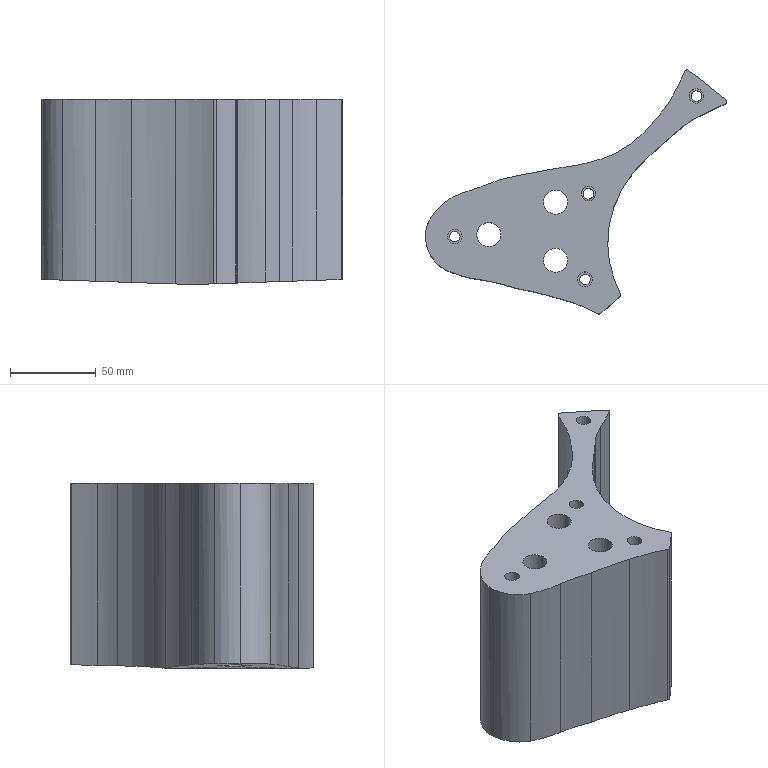Part | NX | features 8 2 | 1 solid | 51 faces | box 175.754 x 142.388 x 108 mm | volume 771641 mm3 | cylinder 37 | plane 14 | commonest cylinder face diameters 3 x4 6.2 x4 8.5 x4 14.1 x3 20 x3 40.451 x1
STEP:
#1=CARTESIAN_POINT('',(739.823,139.747,91.));
#2=VERTEX_POINT('',#1);
#3=CARTESIAN_POINT('',(732.773,139.747,91.));
#4=DIRECTION('',(0.,0.,1.));
#5=DIRECTION('',(1.,0.,0.));
#6=AXIS2_PLACEMENT_3D('',#3,#4,#5);
#7=CIRCLE('',#6,7.05);
#8=EDGE_CURVE('',#2,#2,#7,.T.);
#9=ORIENTED_EDGE('',*,*,#8,.F.);
#10=EDGE_LOOP('',(#9));
#11=FACE_BOUND('',#10,.T.);
#12=CARTESIAN_POINT('',(661.244,132.571,91.));
#13=VERTEX_POINT('',#12);
#14=CARTESIAN_POINT('',(656.895,117.671,91.));
#15=VERTEX_POINT('',#14);
#16=CARTESIAN_POINT('',(676.999,119.888,91.));
#17=DIRECTION('',(0.,0.,1.));
#18=DIRECTION('',(1.,0.,0.));
#19=AXIS2_PLACEMENT_3D('',#16,#17,#18);
#20=CIRCLE('',#19,20.225);
#21=EDGE_CURVE('',#13,#15,#20,.T.);
#22=ORIENTED_EDGE('',*,*,#21,.T.);
#23=CARTESIAN_POINT('',(669.269,99.827,91.));
#24=VERTEX_POINT('',#23);
#25=CARTESIAN_POINT('',(678.925,119.735,91.));
#26=DIRECTION('',(0.,0.,1.));
#27=DIRECTION('',(1.,0.,0.));
#28=AXIS2_PLACEMENT_3D('',#25,#26,#27);
#29=CIRCLE('',#28,22.127);
#30=EDGE_CURVE('',#15,#24,#29,.T.);
#31=ORIENTED_EDGE('',*,*,#30,.T.);
#32=CARTESIAN_POINT('',(688.554,94.53,91.));
#33=VERTEX_POINT('',#32);
#34=CARTESIAN_POINT('',(695.454,157.414,91.));
#35=DIRECTION('',(0.,0.,1.));
#36=DIRECTION('',(1.,0.,0.));
#37=AXIS2_PLACEMENT_3D('',#34,#35,#36);
#38=CIRCLE('',#37,63.261);
#39=EDGE_CURVE('',#24,#33,#38,.T.);
#40=ORIENTED_EDGE('',*,*,#39,.T.);
#41=CARTESIAN_POINT('',(709.333,89.489,91.));
#42=VERTEX_POINT('',#41);
#43=CARTESIAN_POINT('',(668.152,-34.909,91.));
#44=DIRECTION('',(0.,0.,-1.));
#45=DIRECTION('',(1.,0.,0.));
#46=AXIS2_PLACEMENT_3D('',#43,#44,#45);
#47=CIRCLE('',#46,131.038);
#48=EDGE_CURVE('',#33,#42,#47,.T.);
#49=ORIENTED_EDGE('',*,*,#48,.T.);
#50=CARTESIAN_POINT('',(734.802,83.424,91.));
#51=VERTEX_POINT('',#50);
#52=CARTESIAN_POINT('',(672.24,-122.755,91.));
#53=DIRECTION('',(0.,0.,-1.));
#54=DIRECTION('',(1.,0.,0.));
#55=AXIS2_PLACEMENT_3D('',#52,#53,#54);
#56=CIRCLE('',#55,215.461);
#57=EDGE_CURVE('',#42,#51,#56,.T.);
#58=ORIENTED_EDGE('',*,*,#57,.T.);
#59=CARTESIAN_POINT('',(757.492,74.697,91.));
#60=VERTEX_POINT('',#59);
#61=CARTESIAN_POINT('',(709.102,-17.264,91.));
#62=DIRECTION('',(0.,0.,-1.));
#63=DIRECTION('',(1.,0.,0.));
#64=AXIS2_PLACEMENT_3D('',#61,#62,#63);
#65=CIRCLE('',#64,103.916);
#66=EDGE_CURVE('',#51,#60,#65,.T.);
#67=ORIENTED_EDGE('',*,*,#66,.T.);
#68=CARTESIAN_POINT('',(759.172,74.89,91.));
#69=VERTEX_POINT('',#68);
#70=CARTESIAN_POINT('',(758.191,76.024,91.));
#71=DIRECTION('',(0.,0.,1.));
#72=DIRECTION('',(1.,0.,0.));
#73=AXIS2_PLACEMENT_3D('',#70,#71,#72);
#74=CIRCLE('',#73,1.5);
#75=EDGE_CURVE('',#60,#69,#74,.T.);
#76=ORIENTED_EDGE('',*,*,#75,.T.);
#77=CARTESIAN_POINT('',(770.213,84.446,91.));
#78=VERTEX_POINT('',#77);
#79=CARTESIAN_POINT('',(406.095,-230.692,91.));
#80=DIRECTION('',(0.7561,0.6544,0.));
#81=VECTOR('',#80,1000.);
#82=LINE('',#79,#81);
#83=EDGE_CURVE('',#69,#78,#82,.T.);
#84=ORIENTED_EDGE('',*,*,#83,.T.);
#85=CARTESIAN_POINT('',(770.56,86.277,91.));
#86=VERTEX_POINT('',#85);
#87=CARTESIAN_POINT('',(769.232,85.58,91.));
#88=DIRECTION('',(0.,0.,1.));
#89=DIRECTION('',(1.,0.,0.));
#90=AXIS2_PLACEMENT_3D('',#87,#88,#89);
#91=CIRCLE('',#90,1.5);
#92=EDGE_CURVE('',#78,#86,#91,.T.);
#93=ORIENTED_EDGE('',*,*,#92,.T.);
#94=CARTESIAN_POINT('',(763.173,114.849,91.));
#95=VERTEX_POINT('',#94);
#96=CARTESIAN_POINT('',(827.93,116.35,91.));
#97=DIRECTION('',(0.,0.,-1.));
#98=DIRECTION('',(1.,0.,0.));
#99=AXIS2_PLACEMENT_3D('',#96,#97,#98);
#100=CIRCLE('',#99,64.774);
#101=EDGE_CURVE('',#86,#95,#100,.T.);
#102=ORIENTED_EDGE('',*,*,#101,.T.);
#103=CARTESIAN_POINT('',(771.435,147.148,91.));
#104=VERTEX_POINT('',#103);
#105=CARTESIAN_POINT('',(826.446,115.87,91.));
#106=DIRECTION('',(0.,0.,-1.));
#107=DIRECTION('',(1.,0.,0.));
#108=AXIS2_PLACEMENT_3D('',#105,#106,#107);
#109=CIRCLE('',#108,63.281);
#110=EDGE_CURVE('',#95,#104,#109,.T.);
#111=ORIENTED_EDGE('',*,*,#110,.T.);
#112=CARTESIAN_POINT('',(787.822,167.002,91.));
#113=VERTEX_POINT('',#112);
#114=CARTESIAN_POINT('',(839.48,107.677,91.));
#115=DIRECTION('',(0.,0.,-1.));
#116=DIRECTION('',(1.,0.,0.));
#117=AXIS2_PLACEMENT_3D('',#114,#115,#116);
#118=CIRCLE('',#117,78.664);
#119=EDGE_CURVE('',#104,#113,#118,.T.);
#120=ORIENTED_EDGE('',*,*,#119,.T.);
#121=CARTESIAN_POINT('',(795.884,174.026,91.));
#122=VERTEX_POINT('',#121);
#123=CARTESIAN_POINT('',(374.973,-192.67,91.));
#124=DIRECTION('',(0.754,0.6569,0.));
#125=VECTOR('',#124,1000.);
#126=LINE('',#123,#125);
#127=EDGE_CURVE('',#113,#122,#126,.T.);
#128=ORIENTED_EDGE('',*,*,#127,.T.);
#129=CARTESIAN_POINT('',(803.49,180.68,91.));
#130=VERTEX_POINT('',#129);
#131=CARTESIAN_POINT('',(376.367,-192.972,91.));
#132=DIRECTION('',(0.7526,0.6584,0.));
#133=VECTOR('',#132,1000.);
#134=LINE('',#131,#133);
#135=EDGE_CURVE('',#122,#130,#134,.T.);
#136=ORIENTED_EDGE('',*,*,#135,.T.);
#137=CARTESIAN_POINT('',(817.08,190.116,91.));
#138=VERTEX_POINT('',#137);
#139=CARTESIAN_POINT('',(840.917,141.281,91.));
#140=DIRECTION('',(0.,0.,-1.));
#141=DIRECTION('',(1.,0.,0.));
#142=AXIS2_PLACEMENT_3D('',#139,#140,#141);
#143=CIRCLE('',#142,54.342);
#144=EDGE_CURVE('',#130,#138,#143,.T.);
#145=ORIENTED_EDGE('',*,*,#144,.T.);
#146=CARTESIAN_POINT('',(831.695,197.052,91.));
#147=VERTEX_POINT('',#146);
#148=CARTESIAN_POINT('',(632.757,597.362,91.));
#149=DIRECTION('',(0.,0.,1.));
#150=DIRECTION('',(1.,0.,0.));
#151=AXIS2_PLACEMENT_3D('',#148,#149,#150);
#152=CIRCLE('',#151,447.018);
#153=EDGE_CURVE('',#138,#147,#152,.T.);
#154=ORIENTED_EDGE('',*,*,#153,.T.);
#155=CARTESIAN_POINT('',(831.961,199.569,91.));
#156=VERTEX_POINT('',#155);
#157=CARTESIAN_POINT('',(831.027,198.395,91.));
#158=DIRECTION('',(0.,0.,1.));
#159=DIRECTION('',(1.,0.,0.));
#160=AXIS2_PLACEMENT_3D('',#157,#158,#159);
#161=CIRCLE('',#160,1.5);
#162=EDGE_CURVE('',#147,#156,#161,.T.);
#163=ORIENTED_EDGE('',*,*,#162,.T.);
#164=CARTESIAN_POINT('',(810.569,216.587,91.));
#165=VERTEX_POINT('',#164);
#166=CARTESIAN_POINT('',(424.096,524.034,91.));
#167=DIRECTION('',(-0.7826,0.6226,0.));
#168=VECTOR('',#167,1000.);
#169=LINE('',#166,#168);
#170=EDGE_CURVE('',#156,#165,#169,.T.);
#171=ORIENTED_EDGE('',*,*,#170,.T.);
#172=CARTESIAN_POINT('',(808.272,216.04,91.));
#173=VERTEX_POINT('',#172);
#174=CARTESIAN_POINT('',(809.635,215.413,91.));
#175=DIRECTION('',(0.,0.,1.));
#176=DIRECTION('',(1.,0.,0.));
#177=AXIS2_PLACEMENT_3D('',#174,#175,#176);
#178=CIRCLE('',#177,1.5);
#179=EDGE_CURVE('',#165,#173,#178,.T.);
#180=ORIENTED_EDGE('',*,*,#179,.T.);
#181=CARTESIAN_POINT('',(800.673,201.002,91.));
#182=VERTEX_POINT('',#181);
#183=CARTESIAN_POINT('',(597.133,313.29,91.));
#184=DIRECTION('',(0.,0.,-1.));
#185=DIRECTION('',(1.,0.,0.));
#186=AXIS2_PLACEMENT_3D('',#183,#184,#185);
#187=CIRCLE('',#186,232.459);
#188=EDGE_CURVE('',#173,#182,#187,.T.);
#189=ORIENTED_EDGE('',*,*,#188,.T.);
#190=CARTESIAN_POINT('',(792.153,189.249,91.));
#191=VERTEX_POINT('',#190);
#192=CARTESIAN_POINT('',(742.965,233.873,91.));
#193=DIRECTION('',(0.,0.,-1.));
#194=DIRECTION('',(1.,0.,0.));
#195=AXIS2_PLACEMENT_3D('',#192,#193,#194);
#196=CIRCLE('',#195,66.413);
#197=EDGE_CURVE('',#182,#191,#196,.T.);
#198=ORIENTED_EDGE('',*,*,#197,.T.);
#199=CARTESIAN_POINT('',(767.073,167.853,91.));
#200=VERTEX_POINT('',#199);
#201=CARTESIAN_POINT('',(735.807,229.9,91.));
#202=DIRECTION('',(0.,0.,-1.));
#203=DIRECTION('',(1.,0.,0.));
#204=AXIS2_PLACEMENT_3D('',#201,#202,#203);
#205=CIRCLE('',#204,69.48);
#206=EDGE_CURVE('',#191,#200,#205,.T.);
#207=ORIENTED_EDGE('',*,*,#206,.T.);
#208=CARTESIAN_POINT('',(744.942,161.237,91.));
#209=VERTEX_POINT('',#208);
#210=CARTESIAN_POINT('',(729.089,254.594,91.));
#211=DIRECTION('',(0.,0.,-1.));
#212=DIRECTION('',(1.,0.,0.));
#213=AXIS2_PLACEMENT_3D('',#210,#211,#212);
#214=CIRCLE('',#213,94.693);
#215=EDGE_CURVE('',#200,#209,#214,.T.);
#216=ORIENTED_EDGE('',*,*,#215,.T.);
#217=CARTESIAN_POINT('',(699.905,152.757,91.));
#218=VERTEX_POINT('',#217);
#219=CARTESIAN_POINT('',(820.799,-365.438,91.));
#220=DIRECTION('',(0.,0.,1.));
#221=DIRECTION('',(1.,0.,0.));
#222=AXIS2_PLACEMENT_3D('',#219,#220,#221);
#223=CIRCLE('',#222,532.11);
#224=EDGE_CURVE('',#209,#218,#223,.T.);
#225=ORIENTED_EDGE('',*,*,#224,.T.);
#226=CARTESIAN_POINT('',(680.986,145.908,91.));
#227=VERTEX_POINT('',#226);
#228=CARTESIAN_POINT('',(585.955,437.965,91.));
#229=DIRECTION('',(0.,0.,-1.));
#230=DIRECTION('',(1.,0.,0.));
#231=AXIS2_PLACEMENT_3D('',#228,#229,#230);
#232=CIRCLE('',#231,307.129);
#233=EDGE_CURVE('',#218,#227,#232,.T.);
#234=ORIENTED_EDGE('',*,*,#233,.T.);
#235=CARTESIAN_POINT('',(671.706,142.125,91.));
#236=VERTEX_POINT('',#235);
#237=CARTESIAN_POINT('',(693.196,102.677,91.));
#238=DIRECTION('',(0.,0.,1.));
#239=DIRECTION('',(1.,0.,0.));
#240=AXIS2_PLACEMENT_3D('',#237,#238,#239);
#241=CIRCLE('',#240,44.922);
#242=EDGE_CURVE('',#227,#236,#241,.T.);
#243=ORIENTED_EDGE('',*,*,#242,.T.);
#244=CARTESIAN_POINT('',(691.977,109.423,91.));
#245=DIRECTION('',(0.,0.,1.));
#246=DIRECTION('',(1.,0.,0.));
#247=AXIS2_PLACEMENT_3D('',#244,#245,#246);
#248=CIRCLE('',#247,38.475);
#249=EDGE_CURVE('',#236,#13,#248,.T.);
#250=ORIENTED_EDGE('',*,*,#249,.T.);
#251=EDGE_LOOP('',(#22,#31,#40,#49,#58,#67,#76,#84,#93,#102,#111,#120,#128,#136,#145,#154,#163,#171,#180,#189,#198,#207,#216,#225,#234,#243,#250));
#252=FACE_BOUND('',#251,.T.);
#253=CARTESIAN_POINT('',(678.189,119.723,91.));
#254=VERTEX_POINT('',#253);
#255=CARTESIAN_POINT('',(673.939,119.723,91.));
#256=DIRECTION('',(0.,0.,-1.));
#257=DIRECTION('',(1.,0.,0.));
#258=AXIS2_PLACEMENT_3D('',#255,#256,#257);
#259=CIRCLE('',#258,4.25);
#260=EDGE_CURVE('',#254,#254,#259,.T.);
#261=ORIENTED_EDGE('',*,*,#260,.T.);
#262=EDGE_LOOP('',(#261));
#263=FACE_BOUND('',#262,.T.);
#264=CARTESIAN_POINT('',(754.189,94.723,91.));
#265=VERTEX_POINT('',#264);
#266=CARTESIAN_POINT('',(749.939,94.723,91.));
#267=DIRECTION('',(0.,0.,-1.));
#268=DIRECTION('',(1.,0.,0.));
#269=AXIS2_PLACEMENT_3D('',#266,#267,#268);
#270=CIRCLE('',#269,4.25);
#271=EDGE_CURVE('',#265,#265,#270,.T.);
#272=ORIENTED_EDGE('',*,*,#271,.T.);
#273=EDGE_LOOP('',(#272));
#274=FACE_BOUND('',#273,.T.);
#275=CARTESIAN_POINT('',(756.189,144.723,91.));
#276=VERTEX_POINT('',#275);
#277=CARTESIAN_POINT('',(751.939,144.723,91.));
#278=DIRECTION('',(0.,0.,-1.));
#279=DIRECTION('',(1.,0.,0.));
#280=AXIS2_PLACEMENT_3D('',#277,#278,#279);
#281=CIRCLE('',#280,4.25);
#282=EDGE_CURVE('',#276,#276,#281,.T.);
#283=ORIENTED_EDGE('',*,*,#282,.T.);
#284=EDGE_LOOP('',(#283));
#285=FACE_BOUND('',#284,.T.);
#286=CARTESIAN_POINT('',(819.189,201.723,91.));
#287=VERTEX_POINT('',#286);
#288=CARTESIAN_POINT('',(814.939,201.723,91.));
#289=DIRECTION('',(0.,0.,-1.));
#290=DIRECTION('',(1.,0.,0.));
#291=AXIS2_PLACEMENT_3D('',#288,#289,#290);
#292=CIRCLE('',#291,4.25);
#293=EDGE_CURVE('',#287,#287,#292,.T.);
#294=ORIENTED_EDGE('',*,*,#293,.T.);
#295=EDGE_LOOP('',(#294));
#296=FACE_BOUND('',#295,.T.);
#297=CARTESIAN_POINT('',(739.823,105.747,91.));
#298=VERTEX_POINT('',#297);
#299=CARTESIAN_POINT('',(732.773,105.747,91.));
#300=DIRECTION('',(0.,0.,1.));
#301=DIRECTION('',(1.,0.,0.));
#302=AXIS2_PLACEMENT_3D('',#299,#300,#301);
#303=CIRCLE('',#302,7.05);
#304=EDGE_CURVE('',#298,#298,#303,.T.);
#305=ORIENTED_EDGE('',*,*,#304,.F.);
#306=EDGE_LOOP('',(#305));
#307=FACE_BOUND('',#306,.T.);
#308=CARTESIAN_POINT('',(700.823,120.747,91.));
#309=VERTEX_POINT('',#308);
#310=CARTESIAN_POINT('',(693.773,120.747,91.));
#311=DIRECTION('',(0.,0.,1.));
#312=DIRECTION('',(1.,0.,0.));
#313=AXIS2_PLACEMENT_3D('',#310,#311,#312);
#314=CIRCLE('',#313,7.05);
#315=EDGE_CURVE('',#309,#309,#314,.T.);
#316=ORIENTED_EDGE('',*,*,#315,.F.);
#317=EDGE_LOOP('',(#316));
#318=FACE_BOUND('',#317,.T.);
#319=CARTESIAN_POINT('',(102.63,119.939,91.));
#320=DIRECTION('',(0.,0.,1.));
#321=DIRECTION('',(-1.,0.,0.));
#322=AXIS2_PLACEMENT_3D('',#319,#320,#321);
#323=PLANE('',#322);
#324=ADVANCED_FACE('',(#11,#252,#263,#274,#285,#296,#307,#318),#323,.T.);
#325=CARTESIAN_POINT('',(683.773,120.747,-14.918));
#326=VERTEX_POINT('',#325);
#327=CARTESIAN_POINT('',(693.773,120.747,-15.258));
#328=DIRECTION('',(-0.03397,0.,-0.9994));
#329=DIRECTION('',(-0.9994,0.,0.03397));
#330=AXIS2_PLACEMENT_3D('',#327,#328,#329);
#331=ELLIPSE('',#330,10.006,10.);
#332=EDGE_CURVE('',#326,#326,#331,.T.);
#333=ORIENTED_EDGE('',*,*,#332,.F.);
#334=EDGE_LOOP('',(#333));
#335=FACE_BOUND('',#334,.T.);
#336=CARTESIAN_POINT('',(722.773,139.747,-16.243));
#337=VERTEX_POINT('',#336);
#338=CARTESIAN_POINT('',(732.773,139.747,-16.583));
#339=DIRECTION('',(-0.03397,0.,-0.9994));
#340=DIRECTION('',(-0.9994,0.,0.03397));
#341=AXIS2_PLACEMENT_3D('',#338,#339,#340);
#342=ELLIPSE('',#341,10.006,10.);
#343=EDGE_CURVE('',#337,#337,#342,.T.);
#344=ORIENTED_EDGE('',*,*,#343,.F.);
#345=EDGE_LOOP('',(#344));
#346=FACE_BOUND('',#345,.T.);
#347=CARTESIAN_POINT('',(722.773,105.747,-16.243));
#348=VERTEX_POINT('',#347);
#349=CARTESIAN_POINT('',(732.773,105.747,-16.583));
#350=DIRECTION('',(-0.03397,0.,-0.9994));
#351=DIRECTION('',(-0.9994,0.,0.03397));
#352=AXIS2_PLACEMENT_3D('',#349,#350,#351);
#353=ELLIPSE('',#352,10.006,10.);
#354=EDGE_CURVE('',#348,#348,#353,.T.);
#355=ORIENTED_EDGE('',*,*,#354,.F.);
#356=EDGE_LOOP('',(#355));
#357=FACE_BOUND('',#356,.T.);
#358=CARTESIAN_POINT('',(677.039,119.723,-14.689));
#359=VERTEX_POINT('',#358);
#360=CARTESIAN_POINT('',(673.939,119.723,-14.583));
#361=DIRECTION('',(-0.03397,0.,-0.9994));
#362=DIRECTION('',(0.9994,0.,-0.03397));
#363=AXIS2_PLACEMENT_3D('',#360,#361,#362);
#364=ELLIPSE('',#363,3.102,3.1);
#365=EDGE_CURVE('',#359,#359,#364,.T.);
#366=ORIENTED_EDGE('',*,*,#365,.F.);
#367=EDGE_LOOP('',(#366));
#368=FACE_BOUND('',#367,.T.);
#369=CARTESIAN_POINT('',(744.942,161.237,-16.997));
#370=VERTEX_POINT('',#369);
#371=CARTESIAN_POINT('',(745.033,161.253,-17.));
#372=VERTEX_POINT('',#371);
#373=CARTESIAN_POINT('',(729.089,254.594,-16.458));
#374=DIRECTION('',(0.03397,0.,0.9994));
#375=DIRECTION('',(0.9994,0.,-0.03397));
#376=AXIS2_PLACEMENT_3D('',#373,#374,#375);
#377=ELLIPSE('',#376,94.747,94.693);
#378=EDGE_CURVE('',#370,#372,#377,.T.);
#379=ORIENTED_EDGE('',*,*,#378,.T.);
#380=CARTESIAN_POINT('',(745.033,80.242,-17.));
#381=VERTEX_POINT('',#380);
#382=CARTESIAN_POINT('',(745.033,120.747,-17.));
#383=DIRECTION('',(0.,-1.,0.));
#384=VECTOR('',#383,1000.);
#385=LINE('',#382,#384);
#386=EDGE_CURVE('',#372,#381,#385,.T.);
#387=ORIENTED_EDGE('',*,*,#386,.T.);
#388=CARTESIAN_POINT('',(734.802,83.424,-16.652));
#389=VERTEX_POINT('',#388);
#390=CARTESIAN_POINT('',(709.102,-17.264,-15.779));
#391=DIRECTION('',(0.03397,0.,0.9994));
#392=DIRECTION('',(0.9994,0.,-0.03397));
#393=AXIS2_PLACEMENT_3D('',#390,#391,#392);
#394=ELLIPSE('',#393,103.976,103.916);
#395=EDGE_CURVE('',#381,#389,#394,.T.);
#396=ORIENTED_EDGE('',*,*,#395,.T.);
#397=CARTESIAN_POINT('',(709.333,89.489,-15.787));
#398=VERTEX_POINT('',#397);
#399=CARTESIAN_POINT('',(672.24,-122.755,-14.526));
#400=DIRECTION('',(0.03397,0.,0.9994));
#401=DIRECTION('',(0.9994,0.,-0.03397));
#402=AXIS2_PLACEMENT_3D('',#399,#400,#401);
#403=ELLIPSE('',#402,215.585,215.461);
#404=EDGE_CURVE('',#389,#398,#403,.T.);
#405=ORIENTED_EDGE('',*,*,#404,.T.);
#406=CARTESIAN_POINT('',(688.554,94.53,-15.08));
#407=VERTEX_POINT('',#406);
#408=CARTESIAN_POINT('',(668.152,-34.909,-14.387));
#409=DIRECTION('',(0.03397,0.,0.9994));
#410=DIRECTION('',(0.9994,0.,-0.03397));
#411=AXIS2_PLACEMENT_3D('',#408,#409,#410);
#412=ELLIPSE('',#411,131.114,131.038);
#413=EDGE_CURVE('',#398,#407,#412,.T.);
#414=ORIENTED_EDGE('',*,*,#413,.T.);
#415=CARTESIAN_POINT('',(669.269,99.827,-14.425));
#416=VERTEX_POINT('',#415);
#417=CARTESIAN_POINT('',(695.454,157.414,-15.315));
#418=DIRECTION('',(0.03397,0.,0.9994));
#419=DIRECTION('',(0.9994,0.,-0.03397));
#420=AXIS2_PLACEMENT_3D('',#417,#418,#419);
#421=ELLIPSE('',#420,63.297,63.261);
#422=EDGE_CURVE('',#416,#407,#421,.T.);
#423=ORIENTED_EDGE('',*,*,#422,.F.);
#424=CARTESIAN_POINT('',(656.895,117.671,-14.004));
#425=VERTEX_POINT('',#424);
#426=CARTESIAN_POINT('',(678.925,119.735,-14.753));
#427=DIRECTION('',(0.03397,0.,0.9994));
#428=DIRECTION('',(0.9994,0.,-0.03397));
#429=AXIS2_PLACEMENT_3D('',#426,#427,#428);
#430=ELLIPSE('',#429,22.139,22.127);
#431=EDGE_CURVE('',#425,#416,#430,.T.);
#432=ORIENTED_EDGE('',*,*,#431,.F.);
#433=CARTESIAN_POINT('',(661.244,132.571,-14.152));
#434=VERTEX_POINT('',#433);
#435=CARTESIAN_POINT('',(676.999,119.888,-14.687));
#436=DIRECTION('',(0.03397,0.,0.9994));
#437=DIRECTION('',(0.9994,0.,-0.03397));
#438=AXIS2_PLACEMENT_3D('',#435,#436,#437);
#439=ELLIPSE('',#438,20.237,20.225);
#440=EDGE_CURVE('',#434,#425,#439,.T.);
#441=ORIENTED_EDGE('',*,*,#440,.F.);
#442=CARTESIAN_POINT('',(671.706,142.125,-14.508));
#443=VERTEX_POINT('',#442);
#444=CARTESIAN_POINT('',(691.977,109.423,-15.197));
#445=DIRECTION('',(0.03397,0.,0.9994));
#446=DIRECTION('',(0.9994,0.,-0.03397));
#447=AXIS2_PLACEMENT_3D('',#444,#445,#446);
#448=ELLIPSE('',#447,38.497,38.475);
#449=EDGE_CURVE('',#443,#434,#448,.T.);
#450=ORIENTED_EDGE('',*,*,#449,.F.);
#451=CARTESIAN_POINT('',(680.986,145.908,-14.823));
#452=VERTEX_POINT('',#451);
#453=CARTESIAN_POINT('',(693.196,102.677,-15.238));
#454=DIRECTION('',(0.03397,0.,0.9994));
#455=DIRECTION('',(0.9994,0.,-0.03397));
#456=AXIS2_PLACEMENT_3D('',#453,#454,#455);
#457=ELLIPSE('',#456,44.948,44.922);
#458=EDGE_CURVE('',#452,#443,#457,.T.);
#459=ORIENTED_EDGE('',*,*,#458,.F.);
#460=CARTESIAN_POINT('',(699.905,152.757,-15.466));
#461=VERTEX_POINT('',#460);
#462=CARTESIAN_POINT('',(585.955,437.965,-11.593));
#463=DIRECTION('',(0.03397,0.,0.9994));
#464=DIRECTION('',(0.9994,0.,-0.03397));
#465=AXIS2_PLACEMENT_3D('',#462,#463,#464);
#466=ELLIPSE('',#465,307.307,307.129);
#467=EDGE_CURVE('',#452,#461,#466,.T.);
#468=ORIENTED_EDGE('',*,*,#467,.T.);
#469=CARTESIAN_POINT('',(820.799,-365.438,-19.575));
#470=DIRECTION('',(0.03397,0.,0.9994));
#471=DIRECTION('',(0.9994,0.,-0.03397));
#472=AXIS2_PLACEMENT_3D('',#469,#470,#471);
#473=ELLIPSE('',#472,532.417,532.11);
#474=EDGE_CURVE('',#370,#461,#473,.T.);
#475=ORIENTED_EDGE('',*,*,#474,.F.);
#476=EDGE_LOOP('',(#379,#387,#396,#405,#414,#423,#432,#441,#450,#459,#468,#475));
#477=FACE_BOUND('',#476,.T.);
#478=CARTESIAN_POINT('',(700.903,120.747,-15.5));
#479=DIRECTION('',(-0.03397,0.,-0.9994));
#480=DIRECTION('',(0.9994,0.,-0.03397));
#481=AXIS2_PLACEMENT_3D('',#478,#479,#480);
#482=PLANE('',#481);
#483=ADVANCED_FACE('',(#335,#346,#357,#368,#477),#482,.T.);
#484=CARTESIAN_POINT('',(757.492,74.697,-16.576));
#485=VERTEX_POINT('',#484);
#486=CARTESIAN_POINT('',(709.102,-17.264,-18.221));
#487=DIRECTION('',(-0.03397,0.,0.9994));
#488=DIRECTION('',(-0.9994,0.,-0.03397));
#489=AXIS2_PLACEMENT_3D('',#486,#487,#488);
#490=ELLIPSE('',#489,103.976,103.916);
#491=EDGE_CURVE('',#485,#381,#490,.T.);
#492=ORIENTED_EDGE('',*,*,#491,.F.);
#493=CARTESIAN_POINT('',(757.492,74.697,16.));
#494=DIRECTION('',(0.,0.,-1.));
#495=VECTOR('',#494,1000.);
#496=LINE('',#493,#495);
#497=EDGE_CURVE('',#60,#485,#496,.T.);
#498=ORIENTED_EDGE('',*,*,#497,.F.);
#499=ORIENTED_EDGE('',*,*,#66,.F.);
#500=CARTESIAN_POINT('',(734.802,83.424,16.));
#501=DIRECTION('',(0.,0.,-1.));
#502=VECTOR('',#501,1000.);
#503=LINE('',#500,#502);
#504=EDGE_CURVE('',#51,#389,#503,.T.);
#505=ORIENTED_EDGE('',*,*,#504,.T.);
#506=ORIENTED_EDGE('',*,*,#395,.F.);
#507=EDGE_LOOP('',(#492,#498,#499,#505,#506));
#508=FACE_BOUND('',#507,.T.);
#509=CARTESIAN_POINT('',(709.102,-17.264,16.));
#510=DIRECTION('',(0.,0.,-1.));
#511=DIRECTION('',(-1.,0.,0.));
#512=AXIS2_PLACEMENT_3D('',#509,#510,#511);
#513=CYLINDRICAL_SURFACE('',#512,103.916);
#514=ADVANCED_FACE('',(#508),#513,.F.);
#515=ORIENTED_EDGE('',*,*,#497,.T.);
#516=CARTESIAN_POINT('',(759.172,74.89,-16.519));
#517=VERTEX_POINT('',#516);
#518=CARTESIAN_POINT('',(758.191,76.024,-16.553));
#519=DIRECTION('',(-0.03397,0.,0.9994));
#520=DIRECTION('',(-0.9994,0.,-0.03397));
#521=AXIS2_PLACEMENT_3D('',#518,#519,#520);
#522=ELLIPSE('',#521,1.501,1.5);
#523=EDGE_CURVE('',#485,#517,#522,.T.);
#524=ORIENTED_EDGE('',*,*,#523,.T.);
#525=CARTESIAN_POINT('',(759.172,74.89,16.));
#526=DIRECTION('',(0.,0.,-1.));
#527=VECTOR('',#526,1000.);
#528=LINE('',#525,#527);
#529=EDGE_CURVE('',#69,#517,#528,.T.);
#530=ORIENTED_EDGE('',*,*,#529,.F.);
#531=ORIENTED_EDGE('',*,*,#75,.F.);
#532=EDGE_LOOP('',(#515,#524,#530,#531));
#533=FACE_BOUND('',#532,.T.);
#534=CARTESIAN_POINT('',(758.191,76.024,16.));
#535=DIRECTION('',(0.,0.,-1.));
#536=DIRECTION('',(-1.,0.,0.));
#537=AXIS2_PLACEMENT_3D('',#534,#535,#536);
#538=CYLINDRICAL_SURFACE('',#537,1.5);
#539=ADVANCED_FACE('',(#533),#538,.T.);
#540=CARTESIAN_POINT('',(770.213,84.446,-16.144));
#541=VERTEX_POINT('',#540);
#542=CARTESIAN_POINT('',(759.707,75.353,-16.501));
#543=DIRECTION('',(-0.7559,-0.6542,-0.02569));
#544=VECTOR('',#543,1000.);
#545=LINE('',#542,#544);
#546=EDGE_CURVE('',#541,#517,#545,.T.);
#547=ORIENTED_EDGE('',*,*,#546,.F.);
#548=CARTESIAN_POINT('',(770.213,84.446,16.));
#549=DIRECTION('',(0.,0.,-1.));
#550=VECTOR('',#549,1000.);
#551=LINE('',#548,#550);
#552=EDGE_CURVE('',#78,#541,#551,.T.);
#553=ORIENTED_EDGE('',*,*,#552,.F.);
#554=ORIENTED_EDGE('',*,*,#83,.F.);
#555=ORIENTED_EDGE('',*,*,#529,.T.);
#556=EDGE_LOOP('',(#547,#553,#554,#555));
#557=FACE_BOUND('',#556,.T.);
#558=CARTESIAN_POINT('',(759.172,74.89,16.));
#559=DIRECTION('',(-0.6544,0.7561,0.));
#560=DIRECTION('',(-0.7561,-0.6544,0.));
#561=AXIS2_PLACEMENT_3D('',#558,#559,#560);
#562=PLANE('',#561);
#563=ADVANCED_FACE('',(#557),#562,.F.);
#564=ORIENTED_EDGE('',*,*,#552,.T.);
#565=CARTESIAN_POINT('',(770.56,86.277,-16.132));
#566=VERTEX_POINT('',#565);
#567=CARTESIAN_POINT('',(769.232,85.58,-16.177));
#568=DIRECTION('',(-0.03397,0.,0.9994));
#569=DIRECTION('',(-0.9994,0.,-0.03397));
#570=AXIS2_PLACEMENT_3D('',#567,#568,#569);
#571=ELLIPSE('',#570,1.501,1.5);
#572=EDGE_CURVE('',#541,#566,#571,.T.);
#573=ORIENTED_EDGE('',*,*,#572,.T.);
#574=CARTESIAN_POINT('',(770.56,86.277,16.));
#575=DIRECTION('',(0.,0.,-1.));
#576=VECTOR('',#575,1000.);
#577=LINE('',#574,#576);
#578=EDGE_CURVE('',#86,#566,#577,.T.);
#579=ORIENTED_EDGE('',*,*,#578,.F.);
#580=ORIENTED_EDGE('',*,*,#92,.F.);
#581=EDGE_LOOP('',(#564,#573,#579,#580));
#582=FACE_BOUND('',#581,.T.);
#583=CARTESIAN_POINT('',(769.232,85.58,16.));
#584=DIRECTION('',(0.,0.,-1.));
#585=DIRECTION('',(-1.,0.,0.));
#586=AXIS2_PLACEMENT_3D('',#583,#584,#585);
#587=CYLINDRICAL_SURFACE('',#586,1.5);
#588=ADVANCED_FACE('',(#582),#587,.T.);
#589=CARTESIAN_POINT('',(763.173,114.849,-16.383));
#590=VERTEX_POINT('',#589);
#591=CARTESIAN_POINT('',(827.93,116.35,-14.182));
#592=DIRECTION('',(-0.03397,0.,0.9994));
#593=DIRECTION('',(-0.9994,0.,-0.03397));
#594=AXIS2_PLACEMENT_3D('',#591,#592,#593);
#595=ELLIPSE('',#594,64.811,64.774);
#596=EDGE_CURVE('',#590,#566,#595,.T.);
#597=ORIENTED_EDGE('',*,*,#596,.F.);
#598=CARTESIAN_POINT('',(763.173,114.849,16.));
#599=DIRECTION('',(0.,0.,-1.));
#600=VECTOR('',#599,1000.);
#601=LINE('',#598,#600);
#602=EDGE_CURVE('',#95,#590,#601,.T.);
#603=ORIENTED_EDGE('',*,*,#602,.F.);
#604=ORIENTED_EDGE('',*,*,#101,.F.);
#605=ORIENTED_EDGE('',*,*,#578,.T.);
#606=EDGE_LOOP('',(#597,#603,#604,#605));
#607=FACE_BOUND('',#606,.T.);
#608=CARTESIAN_POINT('',(827.93,116.35,16.));
#609=DIRECTION('',(0.,0.,-1.));
#610=DIRECTION('',(-1.,0.,0.));
#611=AXIS2_PLACEMENT_3D('',#608,#609,#610);
#612=CYLINDRICAL_SURFACE('',#611,64.774);
#613=ADVANCED_FACE('',(#607),#612,.F.);
#614=CARTESIAN_POINT('',(771.435,147.148,-16.103));
#615=VERTEX_POINT('',#614);
#616=CARTESIAN_POINT('',(826.446,115.87,-14.233));
#617=DIRECTION('',(-0.03397,0.,0.9994));
#618=DIRECTION('',(-0.9994,0.,-0.03397));
#619=AXIS2_PLACEMENT_3D('',#616,#617,#618);
#620=ELLIPSE('',#619,63.318,63.281);
#621=EDGE_CURVE('',#615,#590,#620,.T.);
#622=ORIENTED_EDGE('',*,*,#621,.F.);
#623=CARTESIAN_POINT('',(771.435,147.148,16.));
#624=DIRECTION('',(0.,0.,-1.));
#625=VECTOR('',#624,1000.);
#626=LINE('',#623,#625);
#627=EDGE_CURVE('',#104,#615,#626,.T.);
#628=ORIENTED_EDGE('',*,*,#627,.F.);
#629=ORIENTED_EDGE('',*,*,#110,.F.);
#630=ORIENTED_EDGE('',*,*,#602,.T.);
#631=EDGE_LOOP('',(#622,#628,#629,#630));
#632=FACE_BOUND('',#631,.T.);
#633=CARTESIAN_POINT('',(826.446,115.87,16.));
#634=DIRECTION('',(0.,0.,-1.));
#635=DIRECTION('',(-1.,0.,0.));
#636=AXIS2_PLACEMENT_3D('',#633,#634,#635);
#637=CYLINDRICAL_SURFACE('',#636,63.281);
#638=ADVANCED_FACE('',(#632),#637,.F.);
#639=CARTESIAN_POINT('',(787.822,167.002,-15.546));
#640=VERTEX_POINT('',#639);
#641=CARTESIAN_POINT('',(839.48,107.677,-13.79));
#642=DIRECTION('',(-0.03397,0.,0.9994));
#643=DIRECTION('',(-0.9994,0.,-0.03397));
#644=AXIS2_PLACEMENT_3D('',#641,#642,#643);
#645=ELLIPSE('',#644,78.71,78.664);
#646=EDGE_CURVE('',#640,#615,#645,.T.);
#647=ORIENTED_EDGE('',*,*,#646,.F.);
#648=CARTESIAN_POINT('',(787.822,167.002,16.));
#649=DIRECTION('',(0.,0.,-1.));
#650=VECTOR('',#649,1000.);
#651=LINE('',#648,#650);
#652=EDGE_CURVE('',#113,#640,#651,.T.);
#653=ORIENTED_EDGE('',*,*,#652,.F.);
#654=ORIENTED_EDGE('',*,*,#119,.F.);
#655=ORIENTED_EDGE('',*,*,#627,.T.);
#656=EDGE_LOOP('',(#647,#653,#654,#655));
#657=FACE_BOUND('',#656,.T.);
#658=CARTESIAN_POINT('',(839.48,107.677,16.));
#659=DIRECTION('',(0.,0.,-1.));
#660=DIRECTION('',(-1.,0.,0.));
#661=AXIS2_PLACEMENT_3D('',#658,#659,#660);
#662=CYLINDRICAL_SURFACE('',#661,78.664);
#663=ADVANCED_FACE('',(#657),#662,.F.);
#664=CARTESIAN_POINT('',(795.884,174.026,-15.272));
#665=VERTEX_POINT('',#664);
#666=CARTESIAN_POINT('',(788.335,167.449,-15.528));
#667=DIRECTION('',(-0.7537,-0.6567,-0.02562));
#668=VECTOR('',#667,1000.);
#669=LINE('',#666,#668);
#670=EDGE_CURVE('',#665,#640,#669,.T.);
#671=ORIENTED_EDGE('',*,*,#670,.F.);
#672=CARTESIAN_POINT('',(795.884,174.026,16.));
#673=DIRECTION('',(0.,0.,-1.));
#674=VECTOR('',#673,1000.);
#675=LINE('',#672,#674);
#676=EDGE_CURVE('',#122,#665,#675,.T.);
#677=ORIENTED_EDGE('',*,*,#676,.F.);
#678=ORIENTED_EDGE('',*,*,#127,.F.);
#679=ORIENTED_EDGE('',*,*,#652,.T.);
#680=EDGE_LOOP('',(#671,#677,#678,#679));
#681=FACE_BOUND('',#680,.T.);
#682=CARTESIAN_POINT('',(787.822,167.002,16.));
#683=DIRECTION('',(-0.6569,0.754,0.));
#684=DIRECTION('',(-0.754,-0.6569,0.));
#685=AXIS2_PLACEMENT_3D('',#682,#683,#684);
#686=PLANE('',#685);
#687=ADVANCED_FACE('',(#681),#686,.F.);
#688=CARTESIAN_POINT('',(803.49,180.68,-15.013));
#689=VERTEX_POINT('',#688);
#690=CARTESIAN_POINT('',(796.39,174.468,-15.254));
#691=DIRECTION('',(-0.7524,-0.6582,-0.02557));
#692=VECTOR('',#691,1000.);
#693=LINE('',#690,#692);
#694=EDGE_CURVE('',#689,#665,#693,.T.);
#695=ORIENTED_EDGE('',*,*,#694,.F.);
#696=CARTESIAN_POINT('',(803.49,180.68,16.));
#697=DIRECTION('',(0.,0.,-1.));
#698=VECTOR('',#697,1000.);
#699=LINE('',#696,#698);
#700=EDGE_CURVE('',#130,#689,#699,.T.);
#701=ORIENTED_EDGE('',*,*,#700,.F.);
#702=ORIENTED_EDGE('',*,*,#135,.F.);
#703=ORIENTED_EDGE('',*,*,#676,.T.);
#704=EDGE_LOOP('',(#695,#701,#702,#703));
#705=FACE_BOUND('',#704,.T.);
#706=CARTESIAN_POINT('',(795.884,174.026,16.));
#707=DIRECTION('',(-0.6584,0.7526,0.));
#708=DIRECTION('',(-0.7526,-0.6584,0.));
#709=AXIS2_PLACEMENT_3D('',#706,#707,#708);
#710=PLANE('',#709);
#711=ADVANCED_FACE('',(#705),#710,.F.);
#712=CARTESIAN_POINT('',(817.08,190.116,-14.551));
#713=VERTEX_POINT('',#712);
#714=CARTESIAN_POINT('',(840.917,141.281,-13.741));
#715=DIRECTION('',(-0.03397,0.,0.9994));
#716=DIRECTION('',(-0.9994,0.,-0.03397));
#717=AXIS2_PLACEMENT_3D('',#714,#715,#716);
#718=ELLIPSE('',#717,54.373,54.342);
#719=EDGE_CURVE('',#713,#689,#718,.T.);
#720=ORIENTED_EDGE('',*,*,#719,.F.);
#721=CARTESIAN_POINT('',(817.08,190.116,16.));
#722=DIRECTION('',(0.,0.,-1.));
#723=VECTOR('',#722,1000.);
#724=LINE('',#721,#723);
#725=EDGE_CURVE('',#138,#713,#724,.T.);
#726=ORIENTED_EDGE('',*,*,#725,.F.);
#727=ORIENTED_EDGE('',*,*,#144,.F.);
#728=ORIENTED_EDGE('',*,*,#700,.T.);
#729=EDGE_LOOP('',(#720,#726,#727,#728));
#730=FACE_BOUND('',#729,.T.);
#731=CARTESIAN_POINT('',(840.917,141.281,16.));
#732=DIRECTION('',(0.,0.,-1.));
#733=DIRECTION('',(-1.,0.,0.));
#734=AXIS2_PLACEMENT_3D('',#731,#732,#733);
#735=CYLINDRICAL_SURFACE('',#734,54.342);
#736=ADVANCED_FACE('',(#730),#735,.F.);
#737=ORIENTED_EDGE('',*,*,#725,.T.);
#738=CARTESIAN_POINT('',(831.695,197.052,-14.054));
#739=VERTEX_POINT('',#738);
#740=CARTESIAN_POINT('',(632.757,597.362,-20.816));
#741=DIRECTION('',(-0.03397,0.,0.9994));
#742=DIRECTION('',(-0.9994,0.,-0.03397));
#743=AXIS2_PLACEMENT_3D('',#740,#741,#742);
#744=ELLIPSE('',#743,447.276,447.018);
#745=EDGE_CURVE('',#713,#739,#744,.T.);
#746=ORIENTED_EDGE('',*,*,#745,.T.);
#747=CARTESIAN_POINT('',(831.695,197.052,16.));
#748=DIRECTION('',(0.,0.,-1.));
#749=VECTOR('',#748,1000.);
#750=LINE('',#747,#749);
#751=EDGE_CURVE('',#147,#739,#750,.T.);
#752=ORIENTED_EDGE('',*,*,#751,.F.);
#753=ORIENTED_EDGE('',*,*,#153,.F.);
#754=EDGE_LOOP('',(#737,#746,#752,#753));
#755=FACE_BOUND('',#754,.T.);
#756=CARTESIAN_POINT('',(632.757,597.362,16.));
#757=DIRECTION('',(0.,0.,-1.));
#758=DIRECTION('',(-1.,0.,0.));
#759=AXIS2_PLACEMENT_3D('',#756,#757,#758);
#760=CYLINDRICAL_SURFACE('',#759,447.018);
#761=ADVANCED_FACE('',(#755),#760,.T.);
#762=ORIENTED_EDGE('',*,*,#751,.T.);
#763=CARTESIAN_POINT('',(831.961,199.569,-14.045));
#764=VERTEX_POINT('',#763);
#765=CARTESIAN_POINT('',(831.027,198.395,-14.077));
#766=DIRECTION('',(-0.03397,0.,0.9994));
#767=DIRECTION('',(-0.9994,0.,-0.03397));
#768=AXIS2_PLACEMENT_3D('',#765,#766,#767);
#769=ELLIPSE('',#768,1.501,1.5);
#770=EDGE_CURVE('',#739,#764,#769,.T.);
#771=ORIENTED_EDGE('',*,*,#770,.T.);
#772=CARTESIAN_POINT('',(831.961,199.569,16.));
#773=DIRECTION('',(0.,0.,-1.));
#774=VECTOR('',#773,1000.);
#775=LINE('',#772,#774);
#776=EDGE_CURVE('',#156,#764,#775,.T.);
#777=ORIENTED_EDGE('',*,*,#776,.F.);
#778=ORIENTED_EDGE('',*,*,#162,.F.);
#779=EDGE_LOOP('',(#762,#771,#777,#778));
#780=FACE_BOUND('',#779,.T.);
#781=CARTESIAN_POINT('',(831.027,198.395,16.));
#782=DIRECTION('',(0.,0.,-1.));
#783=DIRECTION('',(-1.,0.,0.));
#784=AXIS2_PLACEMENT_3D('',#781,#782,#783);
#785=CYLINDRICAL_SURFACE('',#784,1.5);
#786=ADVANCED_FACE('',(#780),#785,.T.);
#787=CARTESIAN_POINT('',(810.569,216.587,-14.772));
#788=VERTEX_POINT('',#787);
#789=CARTESIAN_POINT('',(832.482,199.154,-14.028));
#790=DIRECTION('',(0.7823,-0.6223,0.02659));
#791=VECTOR('',#790,1000.);
#792=LINE('',#789,#791);
#793=EDGE_CURVE('',#788,#764,#792,.T.);
#794=ORIENTED_EDGE('',*,*,#793,.F.);
#795=CARTESIAN_POINT('',(810.569,216.587,16.));
#796=DIRECTION('',(0.,0.,-1.));
#797=VECTOR('',#796,1000.);
#798=LINE('',#795,#797);
#799=EDGE_CURVE('',#165,#788,#798,.T.);
#800=ORIENTED_EDGE('',*,*,#799,.F.);
#801=ORIENTED_EDGE('',*,*,#170,.F.);
#802=ORIENTED_EDGE('',*,*,#776,.T.);
#803=EDGE_LOOP('',(#794,#800,#801,#802));
#804=FACE_BOUND('',#803,.T.);
#805=CARTESIAN_POINT('',(831.961,199.569,16.));
#806=DIRECTION('',(-0.6226,-0.7826,0.));
#807=DIRECTION('',(0.7826,-0.6226,0.));
#808=AXIS2_PLACEMENT_3D('',#805,#806,#807);
#809=PLANE('',#808);
#810=ADVANCED_FACE('',(#804),#809,.F.);
#811=ORIENTED_EDGE('',*,*,#799,.T.);
#812=CARTESIAN_POINT('',(808.272,216.04,-14.85));
#813=VERTEX_POINT('',#812);
#814=CARTESIAN_POINT('',(809.635,215.413,-14.804));
#815=DIRECTION('',(-0.03397,0.,0.9994));
#816=DIRECTION('',(-0.9994,0.,-0.03397));
#817=AXIS2_PLACEMENT_3D('',#814,#815,#816);
#818=ELLIPSE('',#817,1.501,1.5);
#819=EDGE_CURVE('',#788,#813,#818,.T.);
#820=ORIENTED_EDGE('',*,*,#819,.T.);
#821=CARTESIAN_POINT('',(808.272,216.04,16.));
#822=DIRECTION('',(0.,0.,-1.));
#823=VECTOR('',#822,1000.);
#824=LINE('',#821,#823);
#825=EDGE_CURVE('',#173,#813,#824,.T.);
#826=ORIENTED_EDGE('',*,*,#825,.F.);
#827=ORIENTED_EDGE('',*,*,#179,.F.);
#828=EDGE_LOOP('',(#811,#820,#826,#827));
#829=FACE_BOUND('',#828,.T.);
#830=CARTESIAN_POINT('',(809.635,215.413,16.));
#831=DIRECTION('',(0.,0.,-1.));
#832=DIRECTION('',(-1.,0.,0.));
#833=AXIS2_PLACEMENT_3D('',#830,#831,#832);
#834=CYLINDRICAL_SURFACE('',#833,1.5);
#835=ADVANCED_FACE('',(#829),#834,.T.);
#836=CARTESIAN_POINT('',(800.673,201.002,-15.109));
#837=VERTEX_POINT('',#836);
#838=CARTESIAN_POINT('',(597.133,313.29,-22.027));
#839=DIRECTION('',(-0.03397,0.,0.9994));
#840=DIRECTION('',(-0.9994,0.,-0.03397));
#841=AXIS2_PLACEMENT_3D('',#838,#839,#840);
#842=ELLIPSE('',#841,232.594,232.459);
#843=EDGE_CURVE('',#837,#813,#842,.T.);
#844=ORIENTED_EDGE('',*,*,#843,.F.);
#845=CARTESIAN_POINT('',(800.673,201.002,16.));
#846=DIRECTION('',(0.,0.,-1.));
#847=VECTOR('',#846,1000.);
#848=LINE('',#845,#847);
#849=EDGE_CURVE('',#182,#837,#848,.T.);
#850=ORIENTED_EDGE('',*,*,#849,.F.);
#851=ORIENTED_EDGE('',*,*,#188,.F.);
#852=ORIENTED_EDGE('',*,*,#825,.T.);
#853=EDGE_LOOP('',(#844,#850,#851,#852));
#854=FACE_BOUND('',#853,.T.);
#855=CARTESIAN_POINT('',(597.133,313.29,16.));
#856=DIRECTION('',(0.,0.,-1.));
#857=DIRECTION('',(-1.,0.,0.));
#858=AXIS2_PLACEMENT_3D('',#855,#856,#857);
#859=CYLINDRICAL_SURFACE('',#858,232.459);
#860=ADVANCED_FACE('',(#854),#859,.F.);
#861=CARTESIAN_POINT('',(792.153,189.249,-15.398));
#862=VERTEX_POINT('',#861);
#863=CARTESIAN_POINT('',(742.965,233.873,-17.07));
#864=DIRECTION('',(-0.03397,0.,0.9994));
#865=DIRECTION('',(-0.9994,0.,-0.03397));
#866=AXIS2_PLACEMENT_3D('',#863,#864,#865);
#867=ELLIPSE('',#866,66.451,66.413);
#868=EDGE_CURVE('',#862,#837,#867,.T.);
#869=ORIENTED_EDGE('',*,*,#868,.F.);
#870=CARTESIAN_POINT('',(792.153,189.249,16.));
#871=DIRECTION('',(0.,0.,-1.));
#872=VECTOR('',#871,1000.);
#873=LINE('',#870,#872);
#874=EDGE_CURVE('',#191,#862,#873,.T.);
#875=ORIENTED_EDGE('',*,*,#874,.F.);
#876=ORIENTED_EDGE('',*,*,#197,.F.);
#877=ORIENTED_EDGE('',*,*,#849,.T.);
#878=EDGE_LOOP('',(#869,#875,#876,#877));
#879=FACE_BOUND('',#878,.T.);
#880=CARTESIAN_POINT('',(742.965,233.873,16.));
#881=DIRECTION('',(0.,0.,-1.));
#882=DIRECTION('',(-1.,0.,0.));
#883=AXIS2_PLACEMENT_3D('',#880,#881,#882);
#884=CYLINDRICAL_SURFACE('',#883,66.413);
#885=ADVANCED_FACE('',(#879),#884,.F.);
#886=CARTESIAN_POINT('',(767.073,167.853,-16.251));
#887=VERTEX_POINT('',#886);
#888=CARTESIAN_POINT('',(735.807,229.9,-17.314));
#889=DIRECTION('',(-0.03397,0.,0.9994));
#890=DIRECTION('',(-0.9994,0.,-0.03397));
#891=AXIS2_PLACEMENT_3D('',#888,#889,#890);
#892=ELLIPSE('',#891,69.52,69.48);
#893=EDGE_CURVE('',#887,#862,#892,.T.);
#894=ORIENTED_EDGE('',*,*,#893,.F.);
#895=CARTESIAN_POINT('',(767.073,167.853,16.));
#896=DIRECTION('',(0.,0.,-1.));
#897=VECTOR('',#896,1000.);
#898=LINE('',#895,#897);
#899=EDGE_CURVE('',#200,#887,#898,.T.);
#900=ORIENTED_EDGE('',*,*,#899,.F.);
#901=ORIENTED_EDGE('',*,*,#206,.F.);
#902=ORIENTED_EDGE('',*,*,#874,.T.);
#903=EDGE_LOOP('',(#894,#900,#901,#902));
#904=FACE_BOUND('',#903,.T.);
#905=CARTESIAN_POINT('',(735.807,229.9,16.));
#906=DIRECTION('',(0.,0.,-1.));
#907=DIRECTION('',(-1.,0.,0.));
#908=AXIS2_PLACEMENT_3D('',#905,#906,#907);
#909=CYLINDRICAL_SURFACE('',#908,69.48);
#910=ADVANCED_FACE('',(#904),#909,.F.);
#911=CARTESIAN_POINT('',(729.089,254.594,-17.542));
#912=DIRECTION('',(-0.03397,0.,0.9994));
#913=DIRECTION('',(-0.9994,0.,-0.03397));
#914=AXIS2_PLACEMENT_3D('',#911,#912,#913);
#915=ELLIPSE('',#914,94.747,94.693);
#916=EDGE_CURVE('',#372,#887,#915,.T.);
#917=ORIENTED_EDGE('',*,*,#916,.F.);
#918=ORIENTED_EDGE('',*,*,#378,.F.);
#919=CARTESIAN_POINT('',(744.942,161.237,16.));
#920=DIRECTION('',(0.,0.,-1.));
#921=VECTOR('',#920,1000.);
#922=LINE('',#919,#921);
#923=EDGE_CURVE('',#209,#370,#922,.T.);
#924=ORIENTED_EDGE('',*,*,#923,.F.);
#925=ORIENTED_EDGE('',*,*,#215,.F.);
#926=ORIENTED_EDGE('',*,*,#899,.T.);
#927=EDGE_LOOP('',(#917,#918,#924,#925,#926));
#928=FACE_BOUND('',#927,.T.);
#929=CARTESIAN_POINT('',(729.089,254.594,16.));
#930=DIRECTION('',(0.,0.,-1.));
#931=DIRECTION('',(-1.,0.,0.));
#932=AXIS2_PLACEMENT_3D('',#929,#930,#931);
#933=CYLINDRICAL_SURFACE('',#932,94.693);
#934=ADVANCED_FACE('',(#928),#933,.F.);
#935=CARTESIAN_POINT('',(661.244,132.571,16.));
#936=DIRECTION('',(0.,0.,-1.));
#937=VECTOR('',#936,1000.);
#938=LINE('',#935,#937);
#939=EDGE_CURVE('',#13,#434,#938,.T.);
#940=ORIENTED_EDGE('',*,*,#939,.T.);
#941=ORIENTED_EDGE('',*,*,#440,.T.);
#942=CARTESIAN_POINT('',(656.895,117.671,16.));
#943=DIRECTION('',(0.,0.,-1.));
#944=VECTOR('',#943,1000.);
#945=LINE('',#942,#944);
#946=EDGE_CURVE('',#15,#425,#945,.T.);
#947=ORIENTED_EDGE('',*,*,#946,.F.);
#948=ORIENTED_EDGE('',*,*,#21,.F.);
#949=EDGE_LOOP('',(#940,#941,#947,#948));
#950=FACE_BOUND('',#949,.T.);
#951=CARTESIAN_POINT('',(676.999,119.888,16.));
#952=DIRECTION('',(0.,0.,-1.));
#953=DIRECTION('',(-1.,0.,0.));
#954=AXIS2_PLACEMENT_3D('',#951,#952,#953);
#955=CYLINDRICAL_SURFACE('',#954,20.225);
#956=ADVANCED_FACE('',(#950),#955,.T.);
#957=ORIENTED_EDGE('',*,*,#946,.T.);
#958=ORIENTED_EDGE('',*,*,#431,.T.);
#959=CARTESIAN_POINT('',(669.269,99.827,16.));
#960=DIRECTION('',(0.,0.,-1.));
#961=VECTOR('',#960,1000.);
#962=LINE('',#959,#961);
#963=EDGE_CURVE('',#24,#416,#962,.T.);
#964=ORIENTED_EDGE('',*,*,#963,.F.);
#965=ORIENTED_EDGE('',*,*,#30,.F.);
#966=EDGE_LOOP('',(#957,#958,#964,#965));
#967=FACE_BOUND('',#966,.T.);
#968=CARTESIAN_POINT('',(678.925,119.735,16.));
#969=DIRECTION('',(0.,0.,-1.));
#970=DIRECTION('',(-1.,0.,0.));
#971=AXIS2_PLACEMENT_3D('',#968,#969,#970);
#972=CYLINDRICAL_SURFACE('',#971,22.127);
#973=ADVANCED_FACE('',(#967),#972,.T.);
#974=ORIENTED_EDGE('',*,*,#963,.T.);
#975=ORIENTED_EDGE('',*,*,#422,.T.);
#976=CARTESIAN_POINT('',(688.554,94.53,16.));
#977=DIRECTION('',(0.,0.,-1.));
#978=VECTOR('',#977,1000.);
#979=LINE('',#976,#978);
#980=EDGE_CURVE('',#33,#407,#979,.T.);
#981=ORIENTED_EDGE('',*,*,#980,.F.);
#982=ORIENTED_EDGE('',*,*,#39,.F.);
#983=EDGE_LOOP('',(#974,#975,#981,#982));
#984=FACE_BOUND('',#983,.T.);
#985=CARTESIAN_POINT('',(695.454,157.414,16.));
#986=DIRECTION('',(0.,0.,-1.));
#987=DIRECTION('',(-1.,0.,0.));
#988=AXIS2_PLACEMENT_3D('',#985,#986,#987);
#989=CYLINDRICAL_SURFACE('',#988,63.261);
#990=ADVANCED_FACE('',(#984),#989,.T.);
#991=ORIENTED_EDGE('',*,*,#413,.F.);
#992=CARTESIAN_POINT('',(709.333,89.489,16.));
#993=DIRECTION('',(0.,0.,-1.));
#994=VECTOR('',#993,1000.);
#995=LINE('',#992,#994);
#996=EDGE_CURVE('',#42,#398,#995,.T.);
#997=ORIENTED_EDGE('',*,*,#996,.F.);
#998=ORIENTED_EDGE('',*,*,#48,.F.);
#999=ORIENTED_EDGE('',*,*,#980,.T.);
#1000=EDGE_LOOP('',(#991,#997,#998,#999));
#1001=FACE_BOUND('',#1000,.T.);
#1002=CARTESIAN_POINT('',(668.152,-34.909,16.));
#1003=DIRECTION('',(0.,0.,-1.));
#1004=DIRECTION('',(-1.,0.,0.));
#1005=AXIS2_PLACEMENT_3D('',#1002,#1003,#1004);
#1006=CYLINDRICAL_SURFACE('',#1005,131.038);
#1007=ADVANCED_FACE('',(#1001),#1006,.F.);
#1008=ORIENTED_EDGE('',*,*,#404,.F.);
#1009=ORIENTED_EDGE('',*,*,#504,.F.);
#1010=ORIENTED_EDGE('',*,*,#57,.F.);
#1011=ORIENTED_EDGE('',*,*,#996,.T.);
#1012=EDGE_LOOP('',(#1008,#1009,#1010,#1011));
#1013=FACE_BOUND('',#1012,.T.);
#1014=CARTESIAN_POINT('',(672.24,-122.755,16.));
#1015=DIRECTION('',(0.,0.,-1.));
#1016=DIRECTION('',(-1.,0.,0.));
#1017=AXIS2_PLACEMENT_3D('',#1014,#1015,#1016);
#1018=CYLINDRICAL_SURFACE('',#1017,215.461);
#1019=ADVANCED_FACE('',(#1013),#1018,.F.);
#1020=ORIENTED_EDGE('',*,*,#923,.T.);
#1021=ORIENTED_EDGE('',*,*,#474,.T.);
#1022=CARTESIAN_POINT('',(699.905,152.757,16.));
#1023=DIRECTION('',(0.,0.,-1.));
#1024=VECTOR('',#1023,1000.);
#1025=LINE('',#1022,#1024);
#1026=EDGE_CURVE('',#218,#461,#1025,.T.);
#1027=ORIENTED_EDGE('',*,*,#1026,.F.);
#1028=ORIENTED_EDGE('',*,*,#224,.F.);
#1029=EDGE_LOOP('',(#1020,#1021,#1027,#1028));
#1030=FACE_BOUND('',#1029,.T.);
#1031=CARTESIAN_POINT('',(820.799,-365.438,16.));
#1032=DIRECTION('',(0.,0.,-1.));
#1033=DIRECTION('',(-1.,0.,0.));
#1034=AXIS2_PLACEMENT_3D('',#1031,#1032,#1033);
#1035=CYLINDRICAL_SURFACE('',#1034,532.11);
#1036=ADVANCED_FACE('',(#1030),#1035,.T.);
#1037=ORIENTED_EDGE('',*,*,#467,.F.);
#1038=CARTESIAN_POINT('',(680.986,145.908,16.));
#1039=DIRECTION('',(0.,0.,-1.));
#1040=VECTOR('',#1039,1000.);
#1041=LINE('',#1038,#1040);
#1042=EDGE_CURVE('',#227,#452,#1041,.T.);
#1043=ORIENTED_EDGE('',*,*,#1042,.F.);
#1044=ORIENTED_EDGE('',*,*,#233,.F.);
#1045=ORIENTED_EDGE('',*,*,#1026,.T.);
#1046=EDGE_LOOP('',(#1037,#1043,#1044,#1045));
#1047=FACE_BOUND('',#1046,.T.);
#1048=CARTESIAN_POINT('',(585.955,437.965,16.));
#1049=DIRECTION('',(0.,0.,-1.));
#1050=DIRECTION('',(-1.,0.,0.));
#1051=AXIS2_PLACEMENT_3D('',#1048,#1049,#1050);
#1052=CYLINDRICAL_SURFACE('',#1051,307.129);
#1053=ADVANCED_FACE('',(#1047),#1052,.F.);
#1054=ORIENTED_EDGE('',*,*,#1042,.T.);
#1055=ORIENTED_EDGE('',*,*,#458,.T.);
#1056=CARTESIAN_POINT('',(671.706,142.125,16.));
#1057=DIRECTION('',(0.,0.,-1.));
#1058=VECTOR('',#1057,1000.);
#1059=LINE('',#1056,#1058);
#1060=EDGE_CURVE('',#236,#443,#1059,.T.);
#1061=ORIENTED_EDGE('',*,*,#1060,.F.);
#1062=ORIENTED_EDGE('',*,*,#242,.F.);
#1063=EDGE_LOOP('',(#1054,#1055,#1061,#1062));
#1064=FACE_BOUND('',#1063,.T.);
#1065=CARTESIAN_POINT('',(693.196,102.677,16.));
#1066=DIRECTION('',(0.,0.,-1.));
#1067=DIRECTION('',(-1.,0.,0.));
#1068=AXIS2_PLACEMENT_3D('',#1065,#1066,#1067);
#1069=CYLINDRICAL_SURFACE('',#1068,44.922);
#1070=ADVANCED_FACE('',(#1064),#1069,.T.);
#1071=ORIENTED_EDGE('',*,*,#1060,.T.);
#1072=ORIENTED_EDGE('',*,*,#449,.T.);
#1073=ORIENTED_EDGE('',*,*,#939,.F.);
#1074=ORIENTED_EDGE('',*,*,#249,.F.);
#1075=EDGE_LOOP('',(#1071,#1072,#1073,#1074));
#1076=FACE_BOUND('',#1075,.T.);
#1077=CARTESIAN_POINT('',(691.977,109.423,16.));
#1078=DIRECTION('',(0.,0.,-1.));
#1079=DIRECTION('',(-1.,0.,0.));
#1080=AXIS2_PLACEMENT_3D('',#1077,#1078,#1079);
#1081=CYLINDRICAL_SURFACE('',#1080,38.475);
#1082=ADVANCED_FACE('',(#1076),#1081,.T.);
#1083=CARTESIAN_POINT('',(811.839,201.723,-14.729));
#1084=VERTEX_POINT('',#1083);
#1085=CARTESIAN_POINT('',(814.939,201.723,-14.624));
#1086=DIRECTION('',(0.03397,0.,-0.9994));
#1087=DIRECTION('',(-0.9994,0.,-0.03397));
#1088=AXIS2_PLACEMENT_3D('',#1085,#1086,#1087);
#1089=ELLIPSE('',#1088,3.102,3.1);
#1090=EDGE_CURVE('',#1084,#1084,#1089,.T.);
#1091=ORIENTED_EDGE('',*,*,#1090,.F.);
#1092=EDGE_LOOP('',(#1091));
#1093=FACE_BOUND('',#1092,.T.);
#1094=CARTESIAN_POINT('',(748.839,144.723,-16.871));
#1095=VERTEX_POINT('',#1094);
#1096=CARTESIAN_POINT('',(751.939,144.723,-16.765));
#1097=DIRECTION('',(0.03397,0.,-0.9994));
#1098=DIRECTION('',(-0.9994,0.,-0.03397));
#1099=AXIS2_PLACEMENT_3D('',#1096,#1097,#1098);
#1100=ELLIPSE('',#1099,3.102,3.1);
#1101=EDGE_CURVE('',#1095,#1095,#1100,.T.);
#1102=ORIENTED_EDGE('',*,*,#1101,.F.);
#1103=EDGE_LOOP('',(#1102));
#1104=FACE_BOUND('',#1103,.T.);
#1105=CARTESIAN_POINT('',(746.839,94.723,-16.939));
#1106=VERTEX_POINT('',#1105);
#1107=CARTESIAN_POINT('',(749.939,94.723,-16.833));
#1108=DIRECTION('',(0.03397,0.,-0.9994));
#1109=DIRECTION('',(-0.9994,0.,-0.03397));
#1110=AXIS2_PLACEMENT_3D('',#1107,#1108,#1109);
#1111=ELLIPSE('',#1110,3.102,3.1);
#1112=EDGE_CURVE('',#1106,#1106,#1111,.T.);
#1113=ORIENTED_EDGE('',*,*,#1112,.F.);
#1114=EDGE_LOOP('',(#1113));
#1115=FACE_BOUND('',#1114,.T.);
#1116=ORIENTED_EDGE('',*,*,#386,.F.);
#1117=ORIENTED_EDGE('',*,*,#916,.T.);
#1118=ORIENTED_EDGE('',*,*,#893,.T.);
#1119=ORIENTED_EDGE('',*,*,#868,.T.);
#1120=ORIENTED_EDGE('',*,*,#843,.T.);
#1121=ORIENTED_EDGE('',*,*,#819,.F.);
#1122=ORIENTED_EDGE('',*,*,#793,.T.);
#1123=ORIENTED_EDGE('',*,*,#770,.F.);
#1124=ORIENTED_EDGE('',*,*,#745,.F.);
#1125=ORIENTED_EDGE('',*,*,#719,.T.);
#1126=ORIENTED_EDGE('',*,*,#694,.T.);
#1127=ORIENTED_EDGE('',*,*,#670,.T.);
#1128=ORIENTED_EDGE('',*,*,#646,.T.);
#1129=ORIENTED_EDGE('',*,*,#621,.T.);
#1130=ORIENTED_EDGE('',*,*,#596,.T.);
#1131=ORIENTED_EDGE('',*,*,#572,.F.);
#1132=ORIENTED_EDGE('',*,*,#546,.T.);
#1133=ORIENTED_EDGE('',*,*,#523,.F.);
#1134=ORIENTED_EDGE('',*,*,#491,.T.);
#1135=EDGE_LOOP('',(#1116,#1117,#1118,#1119,#1120,#1121,#1122,#1123,#1124,#1125,#1126,#1127,#1128,#1129,#1130,#1131,#1132,#1133,#1134));
#1136=FACE_BOUND('',#1135,.T.);
#1137=CARTESIAN_POINT('',(789.162,145.856,-15.5));
#1138=DIRECTION('',(0.03397,0.,-0.9994));
#1139=DIRECTION('',(0.9994,0.,0.03397));
#1140=AXIS2_PLACEMENT_3D('',#1137,#1138,#1139);
#1141=PLANE('',#1140);
#1142=ADVANCED_FACE('',(#1093,#1104,#1115,#1136),#1141,.T.);
#1143=CARTESIAN_POINT('',(678.189,119.723,18.));
#1144=VERTEX_POINT('',#1143);
#1145=CARTESIAN_POINT('',(673.939,119.723,18.));
#1146=DIRECTION('',(0.,0.,1.));
#1147=DIRECTION('',(1.,0.,0.));
#1148=AXIS2_PLACEMENT_3D('',#1145,#1146,#1147);
#1149=CIRCLE('',#1148,4.25);
#1150=EDGE_CURVE('',#1144,#1144,#1149,.T.);
#1151=ORIENTED_EDGE('',*,*,#1150,.F.);
#1152=EDGE_LOOP('',(#1151));
#1153=FACE_BOUND('',#1152,.T.);
#1154=ORIENTED_EDGE('',*,*,#260,.F.);
#1155=EDGE_LOOP('',(#1154));
#1156=FACE_BOUND('',#1155,.T.);
#1157=CARTESIAN_POINT('',(673.939,119.723,18.));
#1158=DIRECTION('',(0.,0.,1.));
#1159=DIRECTION('',(-1.,0.,0.));
#1160=AXIS2_PLACEMENT_3D('',#1157,#1158,#1159);
#1161=CYLINDRICAL_SURFACE('',#1160,4.25);
#1162=ADVANCED_FACE('',(#1153,#1156),#1161,.F.);
#1163=ORIENTED_EDGE('',*,*,#365,.T.);
#1164=EDGE_LOOP('',(#1163));
#1165=FACE_BOUND('',#1164,.T.);
#1166=CARTESIAN_POINT('',(670.839,119.723,18.));
#1167=VERTEX_POINT('',#1166);
#1168=CARTESIAN_POINT('',(673.939,119.723,18.));
#1169=DIRECTION('',(0.,0.,1.));
#1170=DIRECTION('',(-1.,0.,0.));
#1171=AXIS2_PLACEMENT_3D('',#1168,#1169,#1170);
#1172=CIRCLE('',#1171,3.1);
#1173=EDGE_CURVE('',#1167,#1167,#1172,.T.);
#1174=ORIENTED_EDGE('',*,*,#1173,.T.);
#1175=EDGE_LOOP('',(#1174));
#1176=FACE_BOUND('',#1175,.T.);
#1177=CARTESIAN_POINT('',(673.939,119.723,16.));
#1178=DIRECTION('',(0.,0.,-1.));
#1179=DIRECTION('',(-1.,0.,0.));
#1180=AXIS2_PLACEMENT_3D('',#1177,#1178,#1179);
#1181=CYLINDRICAL_SURFACE('',#1180,3.1);
#1182=ADVANCED_FACE('',(#1165,#1176),#1181,.F.);
#1183=ORIENTED_EDGE('',*,*,#1173,.F.);
#1184=EDGE_LOOP('',(#1183));
#1185=FACE_BOUND('',#1184,.T.);
#1186=ORIENTED_EDGE('',*,*,#1150,.T.);
#1187=EDGE_LOOP('',(#1186));
#1188=FACE_BOUND('',#1187,.T.);
#1189=CARTESIAN_POINT('',(673.939,119.723,18.));
#1190=DIRECTION('',(0.,0.,-1.));
#1191=DIRECTION('',(1.,0.,0.));
#1192=AXIS2_PLACEMENT_3D('',#1189,#1190,#1191);
#1193=PLANE('',#1192);
#1194=ADVANCED_FACE('',(#1185,#1188),#1193,.F.);
#1195=CARTESIAN_POINT('',(754.189,94.723,18.));
#1196=VERTEX_POINT('',#1195);
#1197=CARTESIAN_POINT('',(749.939,94.723,18.));
#1198=DIRECTION('',(0.,0.,1.));
#1199=DIRECTION('',(1.,0.,0.));
#1200=AXIS2_PLACEMENT_3D('',#1197,#1198,#1199);
#1201=CIRCLE('',#1200,4.25);
#1202=EDGE_CURVE('',#1196,#1196,#1201,.T.);
#1203=ORIENTED_EDGE('',*,*,#1202,.F.);
#1204=EDGE_LOOP('',(#1203));
#1205=FACE_BOUND('',#1204,.T.);
#1206=ORIENTED_EDGE('',*,*,#271,.F.);
#1207=EDGE_LOOP('',(#1206));
#1208=FACE_BOUND('',#1207,.T.);
#1209=CARTESIAN_POINT('',(749.939,94.723,18.));
#1210=DIRECTION('',(0.,0.,1.));
#1211=DIRECTION('',(-1.,0.,0.));
#1212=AXIS2_PLACEMENT_3D('',#1209,#1210,#1211);
#1213=CYLINDRICAL_SURFACE('',#1212,4.25);
#1214=ADVANCED_FACE('',(#1205,#1208),#1213,.F.);
#1215=ORIENTED_EDGE('',*,*,#1112,.T.);
#1216=EDGE_LOOP('',(#1215));
#1217=FACE_BOUND('',#1216,.T.);
#1218=CARTESIAN_POINT('',(746.839,94.723,18.));
#1219=VERTEX_POINT('',#1218);
#1220=CARTESIAN_POINT('',(749.939,94.723,18.));
#1221=DIRECTION('',(0.,0.,1.));
#1222=DIRECTION('',(-1.,0.,0.));
#1223=AXIS2_PLACEMENT_3D('',#1220,#1221,#1222);
#1224=CIRCLE('',#1223,3.1);
#1225=EDGE_CURVE('',#1219,#1219,#1224,.T.);
#1226=ORIENTED_EDGE('',*,*,#1225,.T.);
#1227=EDGE_LOOP('',(#1226));
#1228=FACE_BOUND('',#1227,.T.);
#1229=CARTESIAN_POINT('',(749.939,94.723,16.));
#1230=DIRECTION('',(0.,0.,-1.));
#1231=DIRECTION('',(-1.,0.,0.));
#1232=AXIS2_PLACEMENT_3D('',#1229,#1230,#1231);
#1233=CYLINDRICAL_SURFACE('',#1232,3.1);
#1234=ADVANCED_FACE('',(#1217,#1228),#1233,.F.);
#1235=ORIENTED_EDGE('',*,*,#1225,.F.);
#1236=EDGE_LOOP('',(#1235));
#1237=FACE_BOUND('',#1236,.T.);
#1238=ORIENTED_EDGE('',*,*,#1202,.T.);
#1239=EDGE_LOOP('',(#1238));
#1240=FACE_BOUND('',#1239,.T.);
#1241=CARTESIAN_POINT('',(749.939,94.723,18.));
#1242=DIRECTION('',(0.,0.,-1.));
#1243=DIRECTION('',(1.,0.,0.));
#1244=AXIS2_PLACEMENT_3D('',#1241,#1242,#1243);
#1245=PLANE('',#1244);
#1246=ADVANCED_FACE('',(#1237,#1240),#1245,.F.);
#1247=CARTESIAN_POINT('',(756.189,144.723,18.));
#1248=VERTEX_POINT('',#1247);
#1249=CARTESIAN_POINT('',(751.939,144.723,18.));
#1250=DIRECTION('',(0.,0.,1.));
#1251=DIRECTION('',(1.,0.,0.));
#1252=AXIS2_PLACEMENT_3D('',#1249,#1250,#1251);
#1253=CIRCLE('',#1252,4.25);
#1254=EDGE_CURVE('',#1248,#1248,#1253,.T.);
#1255=ORIENTED_EDGE('',*,*,#1254,.F.);
#1256=EDGE_LOOP('',(#1255));
#1257=FACE_BOUND('',#1256,.T.);
#1258=ORIENTED_EDGE('',*,*,#282,.F.);
#1259=EDGE_LOOP('',(#1258));
#1260=FACE_BOUND('',#1259,.T.);
#1261=CARTESIAN_POINT('',(751.939,144.723,18.));
#1262=DIRECTION('',(0.,0.,1.));
#1263=DIRECTION('',(-1.,0.,0.));
#1264=AXIS2_PLACEMENT_3D('',#1261,#1262,#1263);
#1265=CYLINDRICAL_SURFACE('',#1264,4.25);
#1266=ADVANCED_FACE('',(#1257,#1260),#1265,.F.);
#1267=ORIENTED_EDGE('',*,*,#1101,.T.);
#1268=EDGE_LOOP('',(#1267));
#1269=FACE_BOUND('',#1268,.T.);
#1270=CARTESIAN_POINT('',(748.839,144.723,18.));
#1271=VERTEX_POINT('',#1270);
#1272=CARTESIAN_POINT('',(751.939,144.723,18.));
#1273=DIRECTION('',(0.,0.,1.));
#1274=DIRECTION('',(-1.,0.,0.));
#1275=AXIS2_PLACEMENT_3D('',#1272,#1273,#1274);
#1276=CIRCLE('',#1275,3.1);
#1277=EDGE_CURVE('',#1271,#1271,#1276,.T.);
#1278=ORIENTED_EDGE('',*,*,#1277,.T.);
#1279=EDGE_LOOP('',(#1278));
#1280=FACE_BOUND('',#1279,.T.);
#1281=CARTESIAN_POINT('',(751.939,144.723,16.));
#1282=DIRECTION('',(0.,0.,-1.));
#1283=DIRECTION('',(-1.,0.,0.));
#1284=AXIS2_PLACEMENT_3D('',#1281,#1282,#1283);
#1285=CYLINDRICAL_SURFACE('',#1284,3.1);
#1286=ADVANCED_FACE('',(#1269,#1280),#1285,.F.);
#1287=ORIENTED_EDGE('',*,*,#1277,.F.);
#1288=EDGE_LOOP('',(#1287));
#1289=FACE_BOUND('',#1288,.T.);
#1290=ORIENTED_EDGE('',*,*,#1254,.T.);
#1291=EDGE_LOOP('',(#1290));
#1292=FACE_BOUND('',#1291,.T.);
#1293=CARTESIAN_POINT('',(751.939,144.723,18.));
#1294=DIRECTION('',(0.,0.,-1.));
#1295=DIRECTION('',(1.,0.,0.));
#1296=AXIS2_PLACEMENT_3D('',#1293,#1294,#1295);
#1297=PLANE('',#1296);
#1298=ADVANCED_FACE('',(#1289,#1292),#1297,.F.);
#1299=CARTESIAN_POINT('',(819.189,201.723,18.));
#1300=VERTEX_POINT('',#1299);
#1301=CARTESIAN_POINT('',(814.939,201.723,18.));
#1302=DIRECTION('',(0.,0.,1.));
#1303=DIRECTION('',(1.,0.,0.));
#1304=AXIS2_PLACEMENT_3D('',#1301,#1302,#1303);
#1305=CIRCLE('',#1304,4.25);
#1306=EDGE_CURVE('',#1300,#1300,#1305,.T.);
#1307=ORIENTED_EDGE('',*,*,#1306,.F.);
#1308=EDGE_LOOP('',(#1307));
#1309=FACE_BOUND('',#1308,.T.);
#1310=ORIENTED_EDGE('',*,*,#293,.F.);
#1311=EDGE_LOOP('',(#1310));
#1312=FACE_BOUND('',#1311,.T.);
#1313=CARTESIAN_POINT('',(814.939,201.723,18.));
#1314=DIRECTION('',(0.,0.,1.));
#1315=DIRECTION('',(-1.,0.,0.));
#1316=AXIS2_PLACEMENT_3D('',#1313,#1314,#1315);
#1317=CYLINDRICAL_SURFACE('',#1316,4.25);
#1318=ADVANCED_FACE('',(#1309,#1312),#1317,.F.);
#1319=ORIENTED_EDGE('',*,*,#1090,.T.);
#1320=EDGE_LOOP('',(#1319));
#1321=FACE_BOUND('',#1320,.T.);
#1322=CARTESIAN_POINT('',(811.839,201.723,18.));
#1323=VERTEX_POINT('',#1322);
#1324=CARTESIAN_POINT('',(814.939,201.723,18.));
#1325=DIRECTION('',(0.,0.,1.));
#1326=DIRECTION('',(-1.,0.,0.));
#1327=AXIS2_PLACEMENT_3D('',#1324,#1325,#1326);
#1328=CIRCLE('',#1327,3.1);
#1329=EDGE_CURVE('',#1323,#1323,#1328,.T.);
#1330=ORIENTED_EDGE('',*,*,#1329,.T.);
#1331=EDGE_LOOP('',(#1330));
#1332=FACE_BOUND('',#1331,.T.);
#1333=CARTESIAN_POINT('',(814.939,201.723,16.));
#1334=DIRECTION('',(0.,0.,-1.));
#1335=DIRECTION('',(-1.,0.,0.));
#1336=AXIS2_PLACEMENT_3D('',#1333,#1334,#1335);
#1337=CYLINDRICAL_SURFACE('',#1336,3.1);
#1338=ADVANCED_FACE('',(#1321,#1332),#1337,.F.);
#1339=ORIENTED_EDGE('',*,*,#1329,.F.);
#1340=EDGE_LOOP('',(#1339));
#1341=FACE_BOUND('',#1340,.T.);
#1342=ORIENTED_EDGE('',*,*,#1306,.T.);
#1343=EDGE_LOOP('',(#1342));
#1344=FACE_BOUND('',#1343,.T.);
#1345=CARTESIAN_POINT('',(814.939,201.723,18.));
#1346=DIRECTION('',(0.,0.,-1.));
#1347=DIRECTION('',(1.,0.,0.));
#1348=AXIS2_PLACEMENT_3D('',#1345,#1346,#1347);
#1349=PLANE('',#1348);
#1350=ADVANCED_FACE('',(#1341,#1344),#1349,.F.);
#1351=CARTESIAN_POINT('',(739.823,105.747,61.));
#1352=VERTEX_POINT('',#1351);
#1353=CARTESIAN_POINT('',(732.773,105.747,61.));
#1354=DIRECTION('',(0.,0.,-1.));
#1355=DIRECTION('',(1.,0.,0.));
#1356=AXIS2_PLACEMENT_3D('',#1353,#1354,#1355);
#1357=CIRCLE('',#1356,7.05);
#1358=EDGE_CURVE('',#1352,#1352,#1357,.T.);
#1359=ORIENTED_EDGE('',*,*,#1358,.T.);
#1360=EDGE_LOOP('',(#1359));
#1361=FACE_BOUND('',#1360,.T.);
#1362=ORIENTED_EDGE('',*,*,#304,.T.);
#1363=EDGE_LOOP('',(#1362));
#1364=FACE_BOUND('',#1363,.T.);
#1365=CARTESIAN_POINT('',(732.773,105.747,-12.));
#1366=DIRECTION('',(0.,0.,1.));
#1367=DIRECTION('',(-1.,0.,0.));
#1368=AXIS2_PLACEMENT_3D('',#1365,#1366,#1367);
#1369=CYLINDRICAL_SURFACE('',#1368,7.05);
#1370=ADVANCED_FACE('',(#1361,#1364),#1369,.F.);
#1371=ORIENTED_EDGE('',*,*,#1358,.F.);
#1372=EDGE_LOOP('',(#1371));
#1373=FACE_BOUND('',#1372,.T.);
#1374=CARTESIAN_POINT('',(742.773,105.747,61.));
#1375=VERTEX_POINT('',#1374);
#1376=CARTESIAN_POINT('',(732.773,105.747,61.));
#1377=DIRECTION('',(0.,0.,-1.));
#1378=DIRECTION('',(1.,0.,0.));
#1379=AXIS2_PLACEMENT_3D('',#1376,#1377,#1378);
#1380=CIRCLE('',#1379,10.);
#1381=EDGE_CURVE('',#1375,#1375,#1380,.T.);
#1382=ORIENTED_EDGE('',*,*,#1381,.T.);
#1383=EDGE_LOOP('',(#1382));
#1384=FACE_BOUND('',#1383,.T.);
#1385=CARTESIAN_POINT('',(396.279,-423.,61.));
#1386=DIRECTION('',(0.,0.,1.));
#1387=DIRECTION('',(-1.,0.,0.));
#1388=AXIS2_PLACEMENT_3D('',#1385,#1386,#1387);
#1389=PLANE('',#1388);
#1390=ADVANCED_FACE('',(#1373,#1384),#1389,.F.);
#1391=ORIENTED_EDGE('',*,*,#354,.T.);
#1392=EDGE_LOOP('',(#1391));
#1393=FACE_BOUND('',#1392,.T.);
#1394=ORIENTED_EDGE('',*,*,#1381,.F.);
#1395=EDGE_LOOP('',(#1394));
#1396=FACE_BOUND('',#1395,.T.);
#1397=CARTESIAN_POINT('',(732.773,105.747,-12.));
#1398=DIRECTION('',(0.,0.,1.));
#1399=DIRECTION('',(-1.,0.,0.));
#1400=AXIS2_PLACEMENT_3D('',#1397,#1398,#1399);
#1401=CYLINDRICAL_SURFACE('',#1400,10.);
#1402=ADVANCED_FACE('',(#1393,#1396),#1401,.F.);
#1403=CARTESIAN_POINT('',(739.823,139.747,61.));
#1404=VERTEX_POINT('',#1403);
#1405=CARTESIAN_POINT('',(732.773,139.747,61.));
#1406=DIRECTION('',(0.,0.,-1.));
#1407=DIRECTION('',(1.,0.,0.));
#1408=AXIS2_PLACEMENT_3D('',#1405,#1406,#1407);
#1409=CIRCLE('',#1408,7.05);
#1410=EDGE_CURVE('',#1404,#1404,#1409,.T.);
#1411=ORIENTED_EDGE('',*,*,#1410,.T.);
#1412=EDGE_LOOP('',(#1411));
#1413=FACE_BOUND('',#1412,.T.);
#1414=ORIENTED_EDGE('',*,*,#8,.T.);
#1415=EDGE_LOOP('',(#1414));
#1416=FACE_BOUND('',#1415,.T.);
#1417=CARTESIAN_POINT('',(732.773,139.747,-12.));
#1418=DIRECTION('',(0.,0.,1.));
#1419=DIRECTION('',(-1.,0.,0.));
#1420=AXIS2_PLACEMENT_3D('',#1417,#1418,#1419);
#1421=CYLINDRICAL_SURFACE('',#1420,7.05);
#1422=ADVANCED_FACE('',(#1413,#1416),#1421,.F.);
#1423=ORIENTED_EDGE('',*,*,#1410,.F.);
#1424=EDGE_LOOP('',(#1423));
#1425=FACE_BOUND('',#1424,.T.);
#1426=CARTESIAN_POINT('',(742.773,139.747,61.));
#1427=VERTEX_POINT('',#1426);
#1428=CARTESIAN_POINT('',(732.773,139.747,61.));
#1429=DIRECTION('',(0.,0.,-1.));
#1430=DIRECTION('',(1.,0.,0.));
#1431=AXIS2_PLACEMENT_3D('',#1428,#1429,#1430);
#1432=CIRCLE('',#1431,10.);
#1433=EDGE_CURVE('',#1427,#1427,#1432,.T.);
#1434=ORIENTED_EDGE('',*,*,#1433,.T.);
#1435=EDGE_LOOP('',(#1434));
#1436=FACE_BOUND('',#1435,.T.);
#1437=CARTESIAN_POINT('',(396.279,-423.,61.));
#1438=DIRECTION('',(0.,0.,1.));
#1439=DIRECTION('',(-1.,0.,0.));
#1440=AXIS2_PLACEMENT_3D('',#1437,#1438,#1439);
#1441=PLANE('',#1440);
#1442=ADVANCED_FACE('',(#1425,#1436),#1441,.F.);
#1443=ORIENTED_EDGE('',*,*,#343,.T.);
#1444=EDGE_LOOP('',(#1443));
#1445=FACE_BOUND('',#1444,.T.);
#1446=ORIENTED_EDGE('',*,*,#1433,.F.);
#1447=EDGE_LOOP('',(#1446));
#1448=FACE_BOUND('',#1447,.T.);
#1449=CARTESIAN_POINT('',(732.773,139.747,-12.));
#1450=DIRECTION('',(0.,0.,1.));
#1451=DIRECTION('',(-1.,0.,0.));
#1452=AXIS2_PLACEMENT_3D('',#1449,#1450,#1451);
#1453=CYLINDRICAL_SURFACE('',#1452,10.);
#1454=ADVANCED_FACE('',(#1445,#1448),#1453,.F.);
#1455=CARTESIAN_POINT('',(700.823,120.747,61.));
#1456=VERTEX_POINT('',#1455);
#1457=CARTESIAN_POINT('',(693.773,120.747,61.));
#1458=DIRECTION('',(0.,0.,-1.));
#1459=DIRECTION('',(1.,0.,0.));
#1460=AXIS2_PLACEMENT_3D('',#1457,#1458,#1459);
#1461=CIRCLE('',#1460,7.05);
#1462=EDGE_CURVE('',#1456,#1456,#1461,.T.);
#1463=ORIENTED_EDGE('',*,*,#1462,.T.);
#1464=EDGE_LOOP('',(#1463));
#1465=FACE_BOUND('',#1464,.T.);
#1466=ORIENTED_EDGE('',*,*,#315,.T.);
#1467=EDGE_LOOP('',(#1466));
#1468=FACE_BOUND('',#1467,.T.);
#1469=CARTESIAN_POINT('',(693.773,120.747,-12.));
#1470=DIRECTION('',(0.,0.,1.));
#1471=DIRECTION('',(-1.,0.,0.));
#1472=AXIS2_PLACEMENT_3D('',#1469,#1470,#1471);
#1473=CYLINDRICAL_SURFACE('',#1472,7.05);
#1474=ADVANCED_FACE('',(#1465,#1468),#1473,.F.);
#1475=ORIENTED_EDGE('',*,*,#1462,.F.);
#1476=EDGE_LOOP('',(#1475));
#1477=FACE_BOUND('',#1476,.T.);
#1478=CARTESIAN_POINT('',(703.773,120.747,61.));
#1479=VERTEX_POINT('',#1478);
#1480=CARTESIAN_POINT('',(693.773,120.747,61.));
#1481=DIRECTION('',(0.,0.,-1.));
#1482=DIRECTION('',(1.,0.,0.));
#1483=AXIS2_PLACEMENT_3D('',#1480,#1481,#1482);
#1484=CIRCLE('',#1483,10.);
#1485=EDGE_CURVE('',#1479,#1479,#1484,.T.);
#1486=ORIENTED_EDGE('',*,*,#1485,.T.);
#1487=EDGE_LOOP('',(#1486));
#1488=FACE_BOUND('',#1487,.T.);
#1489=CARTESIAN_POINT('',(396.279,-423.,61.));
#1490=DIRECTION('',(0.,0.,1.));
#1491=DIRECTION('',(-1.,0.,0.));
#1492=AXIS2_PLACEMENT_3D('',#1489,#1490,#1491);
#1493=PLANE('',#1492);
#1494=ADVANCED_FACE('',(#1477,#1488),#1493,.F.);
#1495=ORIENTED_EDGE('',*,*,#332,.T.);
#1496=EDGE_LOOP('',(#1495));
#1497=FACE_BOUND('',#1496,.T.);
#1498=ORIENTED_EDGE('',*,*,#1485,.F.);
#1499=EDGE_LOOP('',(#1498));
#1500=FACE_BOUND('',#1499,.T.);
#1501=CARTESIAN_POINT('',(693.773,120.747,-12.));
#1502=DIRECTION('',(0.,0.,1.));
#1503=DIRECTION('',(-1.,0.,0.));
#1504=AXIS2_PLACEMENT_3D('',#1501,#1502,#1503);
#1505=CYLINDRICAL_SURFACE('',#1504,10.);
#1506=ADVANCED_FACE('',(#1497,#1500),#1505,.F.);
#1507=CLOSED_SHELL('',(#324,#483,#514,#539,#563,#588,#613,#638,#663,#687,#711,#736,#761,#786,#810,#835,#860,#885,#910,#934,#956,#973,#990,#1007,#1019,#1036,#1053,#1070,#1082,#1142,#1162,#1182,#1194,#1214,#1234,#1246,#1266,#1286,#1298,#1318,#1338,#1350,#1370,#1390,#1402,#1422,#1442,#1454,#1474,#1494,#1506));
#1508=MANIFOLD_SOLID_BREP('',#1507);
#1509=(LENGTH_UNIT()NAMED_UNIT(*)SI_UNIT(.MILLI.,.METRE.));
#1510=UNCERTAINTY_MEASURE_WITH_UNIT(LENGTH_MEASURE(0.00001),#1509,'','');
#1511=(NAMED_UNIT(*)PLANE_ANGLE_UNIT()SI_UNIT($,.RADIAN.));
#1512=(NAMED_UNIT(*)SI_UNIT($,.STERADIAN.)SOLID_ANGLE_UNIT());
#1513=(GEOMETRIC_REPRESENTATION_CONTEXT(3)GLOBAL_UNCERTAINTY_ASSIGNED_CONTEXT((#1510))GLOBAL_UNIT_ASSIGNED_CONTEXT((#1509,#1511,#1512))REPRESENTATION_CONTEXT('',''));
#1514=ADVANCED_BREP_SHAPE_REPRESENTATION('',(#1508),#1513);